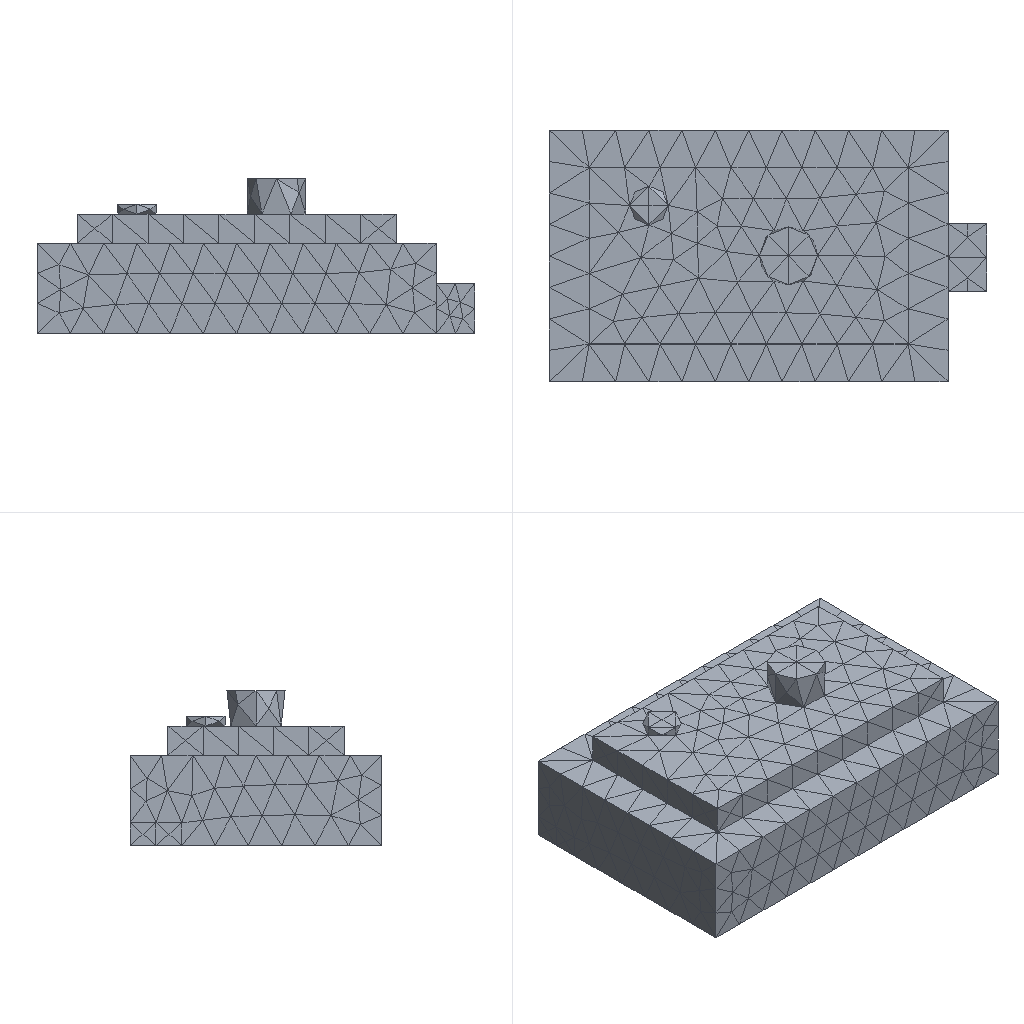Simulation study | ansys mapdl
Set-up summary:
category,name,step,type,value,unit,region
solver,ansys_mapdl
units,mm-N-s-tonne (MPa),,inferred,E=210000 density=
analysis,model,,static
mesh,nodes,,,4143
mesh,elements,,,2409
element_type,SOLID187,,,2409
material,mat 1,,E,210000
material,mat 1,,nu,0.3
load,,model,body load temp,,,all
load,,model,force,"1000 [dir=(0, 0, -1) n=78]",,node list
bc,,model,fixed,"[dofs=UX,UY,UZ n=4621]",,node list
Ansys APDL input file, long lists of numbers shortened:
/COM,ANSYS RELEASE 2026 R1           BUILD 26.1      UP20260202       09:10:33
/PREP7
/NOPR
/TITLE,2
ANTYPE, 0
*IF,_CDRDOFF,EQ,1,THEN     !if solid model was read in
_CDRDOFF=             !reset flag, numoffs already performed
*ELSE              !offset database for the following FE model
NUMOFF,NODE,     4143
NUMOFF,ELEM,     2409
NUMOFF,MAT ,        1
NUMOFF,TYPE,        1
*ENDIF
*SET,_RETURN ,  0.
*SET,_STATUS ,  0.
*SET,_UIQR   ,  78.
*SET,__FLOATPARAMETER__,  4143.
DOF,DELETE
ETBLOCK,        1,        1
(2i9,19a9)
        1      187        0        0        0        0        0        0        0        0        0        0        0        0        0        0        0        0        0        0        0
       -1
NBLOCK,6,SOLID,      4143,      4143
(3i9,6e21.13e3)
        1        0        0-4.5800000000000E+001 3.9000000000000E+001 7.0000000000000E+000
! (4142 more lines like these left out)
N,UNBL,LOC,       -1,
EBLOCK,19,SOLID,      2409,      2409
(19i10)
         1         1         1         1         0         0         0         0        10         0         1      1759      1760      1761      1525      1966      1967      1968      1969
! (4817 more lines like these left out)
        -1
MPTEMP,UNBL, 1, 1,  0.    ,
MPDATA,UNBL, 1,EX  ,       1, 1,  210000.000    ,
MPTEMP,UNBL, 1, 1,  0.    ,
MPDATA,UNBL, 1,NUXY,       1, 1, 0.3    ,
MPTEMP,UNBL, 1, 1,  0.    ,
MPDATA,UNBL, 1,PRXY,       1, 1, 0.3    ,
EXTOPT,ATTR,      0,      0,      0
EXTOPT,ESIZE,  0,  0.
EXTOPT,ACLEAR,      0
TREF,  0.
IRLF,  0
BFUNIF,TEMP,_TINY
ACEL,  0.    ,  0.    ,  0.
OMEGA,  0.    ,  0.    ,  0.
DOMEGA,  0.    ,  0.    ,  0.
CGLOC,  0.    ,  0.    ,  0.
CGOMEGA,  0.    ,  0.    ,  0.
DCGOMG,  0.    ,  0.    ,  0.
KUSE,     0
TIME,  0.
ALPHAD,  0.
BETAD,  0.
DMPRAT,  0.
DMPSTR,  0.
CRPLIM, 0.1    ,   0
CRPLIM,  0.    ,   1
NCNV,     0, 1.000000000E+12,     0,  0.    ,  0.
NEQIT,     0
ERESX,DEFA
DBLOCK,      4621
(i9,a6,2(pg16.9))
        1  UX    0.00000000      0.00000000
! (4620 more lines like these left out)
       -1
FBLOCK,        78
(i9,a6,2(pg16.9))
      845  FZ   -12.8205128      0.00000000
! (77 more lines like these left out)
       -1
/GO
FINISH
Results summary:
result,analysis_type_db,,,static,unstated
result,n_sets,,,1,unstated
result,load_steps[0].set,load_step=1,,1,unstated
result,load_steps[0].substep,load_step=1,,1,unstated
result,load_steps[0].time,load_step=1,,1,unstated
result,load_steps[0].freq,load_step=1,,1,unstated
result,load_steps[0].max_usum,load_step=1,,0.0003494,unstated
result,load_steps[0].max_seqv,load_step=1,,4.914,unstated
result,load_steps[0].reaction_sum.FX,load_step=1,,-1.56639e-11,unstated
result,load_steps[0].reaction_sum.FY,load_step=1,,4.77485e-12,unstated
result,load_steps[0].reaction_sum.FZ,load_step=1,,1000,unstated
result,load_steps[0].reaction_sum.MX,load_step=1,,0,unstated
result,load_steps[0].reaction_sum.MY,load_step=1,,0,unstated
result,load_steps[0].reaction_sum.MZ,load_step=1,,0,unstated
result,convergence,,,results present for all listed sets,unstated